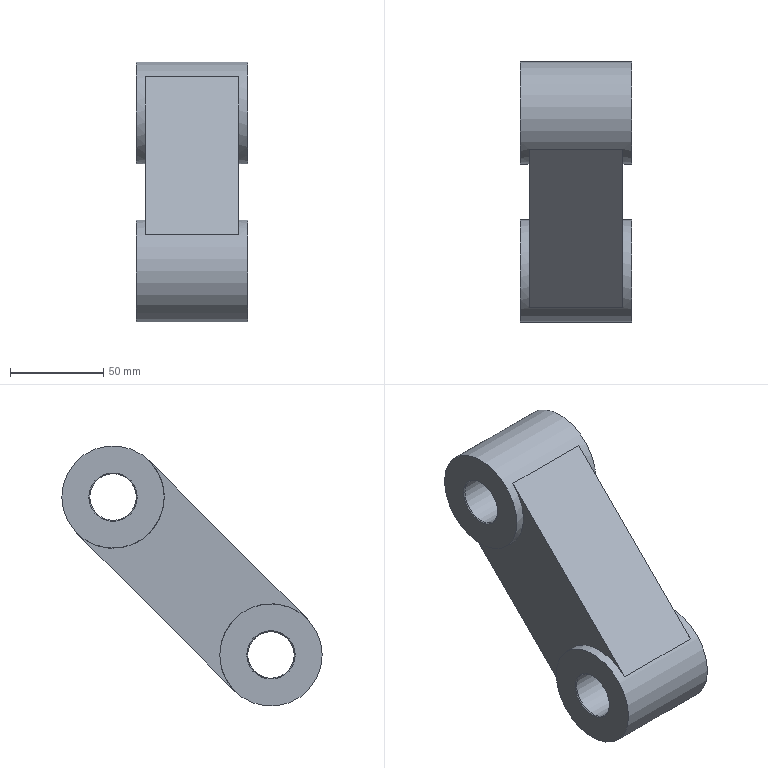Part | NX | features solid 2 | 1 solid | 19 faces | box 60 x 139.853 x 139.853 mm | volume 437363 mm3 | plane 8 | cone 7 | cylinder 4 | commonest cylinder face diameters 25 x2 55 x2
STEP:
#1=CARTESIAN_POINT('',(525.,-759.445,-230.555));
#2=VERTEX_POINT('',#1);
#3=CARTESIAN_POINT('',(475.,-759.445,-230.555));
#4=VERTEX_POINT('',#3);
#5=CARTESIAN_POINT('',(525.,-759.445,-230.555));
#6=DIRECTION('',(-1.,0.,0.));
#7=VECTOR('',#6,1000.);
#8=LINE('',#5,#7);
#9=EDGE_CURVE('',#2,#4,#8,.T.);
#10=ORIENTED_EDGE('',*,*,#9,.F.);
#11=CARTESIAN_POINT('',(525.,-674.593,-145.702));
#12=VERTEX_POINT('',#11);
#13=CARTESIAN_POINT('',(525.,-759.445,-230.555));
#14=DIRECTION('',(0.,0.7071,0.7071));
#15=VECTOR('',#14,1000.);
#16=LINE('',#13,#15);
#17=EDGE_CURVE('',#2,#12,#16,.T.);
#18=ORIENTED_EDGE('',*,*,#17,.T.);
#19=CARTESIAN_POINT('',(475.,-674.593,-145.702));
#20=VERTEX_POINT('',#19);
#21=CARTESIAN_POINT('',(525.,-674.593,-145.702));
#22=DIRECTION('',(-1.,0.,0.));
#23=VECTOR('',#22,1000.);
#24=LINE('',#21,#23);
#25=EDGE_CURVE('',#12,#20,#24,.T.);
#26=ORIENTED_EDGE('',*,*,#25,.T.);
#27=CARTESIAN_POINT('',(475.,-717.019,-188.128));
#28=DIRECTION('',(0.,0.7071,0.7071));
#29=VECTOR('',#28,1000.);
#30=LINE('',#27,#29);
#31=EDGE_CURVE('',#4,#20,#30,.T.);
#32=ORIENTED_EDGE('',*,*,#31,.F.);
#33=EDGE_LOOP('',(#10,#18,#26,#32));
#34=FACE_BOUND('',#33,.T.);
#35=CARTESIAN_POINT('',(575.,-778.891,-250.));
#36=DIRECTION('',(0.,-0.7071,0.7071));
#37=DIRECTION('',(0.,0.7071,0.7071));
#38=AXIS2_PLACEMENT_3D('',#35,#36,#37);
#39=PLANE('',#38);
#40=ADVANCED_FACE('',(#34),#39,.T.);
#41=CARTESIAN_POINT('',(470.,-712.5,-250.));
#42=VERTEX_POINT('',#41);
#43=CARTESIAN_POINT('',(470.,-740.,-250.));
#44=DIRECTION('',(1.,0.,0.));
#45=DIRECTION('',(0.,1.,0.));
#46=AXIS2_PLACEMENT_3D('',#43,#44,#45);
#47=CIRCLE('',#46,27.5);
#48=EDGE_CURVE('',#42,#42,#47,.T.);
#49=ORIENTED_EDGE('',*,*,#48,.T.);
#50=EDGE_LOOP('',(#49));
#51=FACE_BOUND('',#50,.T.);
#52=CARTESIAN_POINT('',(530.,-712.5,-250.));
#53=VERTEX_POINT('',#52);
#54=CARTESIAN_POINT('',(530.,-740.,-250.));
#55=DIRECTION('',(1.,0.,0.));
#56=DIRECTION('',(0.,1.,0.));
#57=AXIS2_PLACEMENT_3D('',#54,#55,#56);
#58=CIRCLE('',#57,27.5);
#59=EDGE_CURVE('',#53,#53,#58,.T.);
#60=ORIENTED_EDGE('',*,*,#59,.F.);
#61=EDGE_LOOP('',(#60));
#62=FACE_BOUND('',#61,.T.);
#63=CARTESIAN_POINT('',(475.,-720.555,-269.445));
#64=VERTEX_POINT('',#63);
#65=CARTESIAN_POINT('',(475.,-740.,-250.));
#66=DIRECTION('',(1.,0.,0.));
#67=DIRECTION('',(0.,1.,0.));
#68=AXIS2_PLACEMENT_3D('',#65,#66,#67);
#69=CIRCLE('',#68,27.5);
#70=EDGE_CURVE('',#64,#4,#69,.T.);
#71=ORIENTED_EDGE('',*,*,#70,.F.);
#72=CARTESIAN_POINT('',(525.,-720.555,-269.445));
#73=VERTEX_POINT('',#72);
#74=CARTESIAN_POINT('',(500.005,-720.555,-269.445));
#75=DIRECTION('',(-1.,0.,0.));
#76=VECTOR('',#75,1000.);
#77=LINE('',#74,#76);
#78=EDGE_CURVE('',#73,#64,#77,.T.);
#79=ORIENTED_EDGE('',*,*,#78,.F.);
#80=CARTESIAN_POINT('',(525.,-740.,-250.));
#81=DIRECTION('',(-1.,0.,0.));
#82=DIRECTION('',(0.,1.,0.));
#83=AXIS2_PLACEMENT_3D('',#80,#81,#82);
#84=CIRCLE('',#83,27.5);
#85=EDGE_CURVE('',#2,#73,#84,.T.);
#86=ORIENTED_EDGE('',*,*,#85,.F.);
#87=ORIENTED_EDGE('',*,*,#9,.T.);
#88=EDGE_LOOP('',(#71,#79,#86,#87));
#89=FACE_BOUND('',#88,.T.);
#90=CARTESIAN_POINT('',(530.106,-740.,-250.));
#91=DIRECTION('',(-1.,0.,0.));
#92=DIRECTION('',(0.,0.,-1.));
#93=AXIS2_PLACEMENT_3D('',#90,#91,#92);
#94=CYLINDRICAL_SURFACE('',#93,27.5);
#95=ADVANCED_FACE('',(#51,#62,#89),#94,.T.);
#96=CARTESIAN_POINT('',(525.,-635.702,-184.593));
#97=VERTEX_POINT('',#96);
#98=CARTESIAN_POINT('',(525.,-678.128,-227.019));
#99=DIRECTION('',(0.,-0.7071,-0.7071));
#100=VECTOR('',#99,1000.);
#101=LINE('',#98,#100);
#102=EDGE_CURVE('',#97,#73,#101,.T.);
#103=ORIENTED_EDGE('',*,*,#102,.T.);
#104=ORIENTED_EDGE('',*,*,#78,.T.);
#105=CARTESIAN_POINT('',(475.,-635.702,-184.593));
#106=VERTEX_POINT('',#105);
#107=CARTESIAN_POINT('',(475.,-678.128,-227.019));
#108=DIRECTION('',(0.,-0.7071,-0.7071));
#109=VECTOR('',#108,1000.);
#110=LINE('',#107,#109);
#111=EDGE_CURVE('',#106,#64,#110,.T.);
#112=ORIENTED_EDGE('',*,*,#111,.F.);
#113=CARTESIAN_POINT('',(500.,-635.702,-184.593));
#114=DIRECTION('',(-1.,0.,0.));
#115=VECTOR('',#114,1000.);
#116=LINE('',#113,#115);
#117=EDGE_CURVE('',#97,#106,#116,.T.);
#118=ORIENTED_EDGE('',*,*,#117,.F.);
#119=EDGE_LOOP('',(#103,#104,#112,#118));
#120=FACE_BOUND('',#119,.T.);
#121=CARTESIAN_POINT('',(575.,-616.256,-165.147));
#122=DIRECTION('',(0.,0.7071,-0.7071));
#123=DIRECTION('',(0.,-0.7071,-0.7071));
#124=AXIS2_PLACEMENT_3D('',#121,#122,#123);
#125=PLANE('',#124);
#126=ADVANCED_FACE('',(#120),#125,.T.);
#127=CARTESIAN_POINT('',(525.,-655.147,-165.147));
#128=DIRECTION('',(-1.,0.,0.));
#129=DIRECTION('',(0.,1.,0.));
#130=AXIS2_PLACEMENT_3D('',#127,#128,#129);
#131=CIRCLE('',#130,27.5);
#132=EDGE_CURVE('',#97,#12,#131,.T.);
#133=ORIENTED_EDGE('',*,*,#132,.F.);
#134=ORIENTED_EDGE('',*,*,#117,.T.);
#135=CARTESIAN_POINT('',(475.,-655.147,-165.147));
#136=DIRECTION('',(1.,0.,0.));
#137=DIRECTION('',(0.,1.,0.));
#138=AXIS2_PLACEMENT_3D('',#135,#136,#137);
#139=CIRCLE('',#138,27.5);
#140=EDGE_CURVE('',#20,#106,#139,.T.);
#141=ORIENTED_EDGE('',*,*,#140,.F.);
#142=ORIENTED_EDGE('',*,*,#25,.F.);
#143=EDGE_LOOP('',(#133,#134,#141,#142));
#144=FACE_BOUND('',#143,.T.);
#145=CARTESIAN_POINT('',(470.,-627.647,-165.147));
#146=VERTEX_POINT('',#145);
#147=CARTESIAN_POINT('',(470.,-655.147,-165.147));
#148=DIRECTION('',(1.,0.,0.));
#149=DIRECTION('',(0.,1.,0.));
#150=AXIS2_PLACEMENT_3D('',#147,#148,#149);
#151=CIRCLE('',#150,27.5);
#152=EDGE_CURVE('',#146,#146,#151,.T.);
#153=ORIENTED_EDGE('',*,*,#152,.T.);
#154=EDGE_LOOP('',(#153));
#155=FACE_BOUND('',#154,.T.);
#156=CARTESIAN_POINT('',(530.,-627.647,-165.147));
#157=VERTEX_POINT('',#156);
#158=CARTESIAN_POINT('',(530.,-655.147,-165.147));
#159=DIRECTION('',(1.,0.,0.));
#160=DIRECTION('',(0.,1.,0.));
#161=AXIS2_PLACEMENT_3D('',#158,#159,#160);
#162=CIRCLE('',#161,27.5);
#163=EDGE_CURVE('',#157,#157,#162,.T.);
#164=ORIENTED_EDGE('',*,*,#163,.F.);
#165=EDGE_LOOP('',(#164));
#166=FACE_BOUND('',#165,.T.);
#167=CARTESIAN_POINT('',(530.106,-655.147,-165.147));
#168=DIRECTION('',(-1.,0.,0.));
#169=DIRECTION('',(0.,0.,-1.));
#170=AXIS2_PLACEMENT_3D('',#167,#168,#169);
#171=CYLINDRICAL_SURFACE('',#170,27.5);
#172=ADVANCED_FACE('',(#144,#155,#166),#171,.T.);
#173=ORIENTED_EDGE('',*,*,#17,.F.);
#174=ORIENTED_EDGE('',*,*,#85,.T.);
#175=ORIENTED_EDGE('',*,*,#102,.F.);
#176=ORIENTED_EDGE('',*,*,#132,.T.);
#177=EDGE_LOOP('',(#173,#174,#175,#176));
#178=FACE_BOUND('',#177,.T.);
#179=CARTESIAN_POINT('',(525.,-707.705,-134.764));
#180=DIRECTION('',(-1.,0.,0.));
#181=DIRECTION('',(0.,0.,-1.));
#182=AXIS2_PLACEMENT_3D('',#179,#180,#181);
#183=PLANE('',#182);
#184=ADVANCED_FACE('',(#178),#183,.F.);
#185=ORIENTED_EDGE('',*,*,#48,.F.);
#186=EDGE_LOOP('',(#185));
#187=FACE_BOUND('',#186,.T.);
#188=CARTESIAN_POINT('',(470.,-727.,-250.));
#189=VERTEX_POINT('',#188);
#190=CARTESIAN_POINT('',(470.,-753.,-250.));
#191=VERTEX_POINT('',#190);
#192=CARTESIAN_POINT('',(470.,-740.,-250.));
#193=DIRECTION('',(1.,0.,0.));
#194=DIRECTION('',(0.,0.,-1.));
#195=AXIS2_PLACEMENT_3D('',#192,#193,#194);
#196=CIRCLE('',#195,13.);
#197=EDGE_CURVE('',#189,#191,#196,.T.);
#198=ORIENTED_EDGE('',*,*,#197,.T.);
#199=CARTESIAN_POINT('',(470.,-740.,-250.));
#200=DIRECTION('',(1.,0.,0.));
#201=DIRECTION('',(0.,0.,-1.));
#202=AXIS2_PLACEMENT_3D('',#199,#200,#201);
#203=CIRCLE('',#202,13.);
#204=EDGE_CURVE('',#191,#189,#203,.T.);
#205=ORIENTED_EDGE('',*,*,#204,.T.);
#206=EDGE_LOOP('',(#198,#205));
#207=FACE_BOUND('',#206,.T.);
#208=CARTESIAN_POINT('',(470.,-743.7,-355.311));
#209=DIRECTION('',(-1.,0.,0.));
#210=DIRECTION('',(0.,0.,-1.));
#211=AXIS2_PLACEMENT_3D('',#208,#209,#210);
#212=PLANE('',#211);
#213=ADVANCED_FACE('',(#187,#207),#212,.T.);
#214=CARTESIAN_POINT('',(470.5,-727.5,-250.));
#215=VERTEX_POINT('',#214);
#216=CARTESIAN_POINT('',(470.244,-727.244,-250.));
#217=DIRECTION('',(-0.7071,0.7071,0.));
#218=VECTOR('',#217,1000.);
#219=LINE('',#216,#218);
#220=EDGE_CURVE('',#215,#189,#219,.T.);
#221=ORIENTED_EDGE('',*,*,#220,.F.);
#222=CARTESIAN_POINT('',(470.5,-752.5,-250.));
#223=VERTEX_POINT('',#222);
#224=CARTESIAN_POINT('',(470.5,-740.,-250.));
#225=DIRECTION('',(-1.,0.,0.));
#226=DIRECTION('',(0.,0.,1.));
#227=AXIS2_PLACEMENT_3D('',#224,#225,#226);
#228=CIRCLE('',#227,12.5);
#229=EDGE_CURVE('',#215,#223,#228,.F.);
#230=ORIENTED_EDGE('',*,*,#229,.T.);
#231=CARTESIAN_POINT('',(470.244,-752.756,-250.));
#232=DIRECTION('',(-0.7071,-0.7071,0.));
#233=VECTOR('',#232,1000.);
#234=LINE('',#231,#233);
#235=EDGE_CURVE('',#191,#223,#234,.F.);
#236=ORIENTED_EDGE('',*,*,#235,.F.);
#237=ORIENTED_EDGE('',*,*,#197,.F.);
#238=EDGE_LOOP('',(#221,#230,#236,#237));
#239=FACE_BOUND('',#238,.T.);
#240=CARTESIAN_POINT('',(470.566,-740.,-250.));
#241=DIRECTION('',(-1.,0.,0.));
#242=DIRECTION('',(0.,0.,-1.));
#243=AXIS2_PLACEMENT_3D('',#240,#241,#242);
#244=CONICAL_SURFACE('',#243,12.434,0.7854);
#245=ADVANCED_FACE('',(#239),#244,.F.);
#246=CARTESIAN_POINT('',(470.5,-740.,-250.));
#247=DIRECTION('',(-1.,0.,0.));
#248=DIRECTION('',(0.,0.,1.));
#249=AXIS2_PLACEMENT_3D('',#246,#247,#248);
#250=CIRCLE('',#249,12.5);
#251=EDGE_CURVE('',#223,#215,#250,.F.);
#252=ORIENTED_EDGE('',*,*,#251,.T.);
#253=ORIENTED_EDGE('',*,*,#220,.T.);
#254=ORIENTED_EDGE('',*,*,#204,.F.);
#255=ORIENTED_EDGE('',*,*,#235,.T.);
#256=EDGE_LOOP('',(#252,#253,#254,#255));
#257=FACE_BOUND('',#256,.T.);
#258=CARTESIAN_POINT('',(470.566,-740.,-250.));
#259=DIRECTION('',(-1.,0.,0.));
#260=DIRECTION('',(0.,0.,-1.));
#261=AXIS2_PLACEMENT_3D('',#258,#259,#260);
#262=CONICAL_SURFACE('',#261,12.434,0.7854);
#263=ADVANCED_FACE('',(#257),#262,.F.);
#264=ORIENTED_EDGE('',*,*,#31,.T.);
#265=ORIENTED_EDGE('',*,*,#140,.T.);
#266=ORIENTED_EDGE('',*,*,#111,.T.);
#267=ORIENTED_EDGE('',*,*,#70,.T.);
#268=EDGE_LOOP('',(#264,#265,#266,#267));
#269=FACE_BOUND('',#268,.T.);
#270=CARTESIAN_POINT('',(475.,-707.705,-134.764));
#271=DIRECTION('',(-1.,0.,0.));
#272=DIRECTION('',(0.,0.,-1.));
#273=AXIS2_PLACEMENT_3D('',#270,#271,#272);
#274=PLANE('',#273);
#275=ADVANCED_FACE('',(#269),#274,.T.);
#276=ORIENTED_EDGE('',*,*,#163,.T.);
#277=EDGE_LOOP('',(#276));
#278=FACE_BOUND('',#277,.T.);
#279=CARTESIAN_POINT('',(530.,-668.147,-165.147));
#280=VERTEX_POINT('',#279);
#281=CARTESIAN_POINT('',(530.,-642.147,-165.147));
#282=VERTEX_POINT('',#281);
#283=CARTESIAN_POINT('',(530.,-655.147,-165.147));
#284=DIRECTION('',(-1.,0.,0.));
#285=DIRECTION('',(0.,0.,1.));
#286=AXIS2_PLACEMENT_3D('',#283,#284,#285);
#287=CIRCLE('',#286,13.);
#288=EDGE_CURVE('',#280,#282,#287,.T.);
#289=ORIENTED_EDGE('',*,*,#288,.T.);
#290=CARTESIAN_POINT('',(530.,-655.147,-165.147));
#291=DIRECTION('',(-1.,0.,0.));
#292=DIRECTION('',(0.,0.,1.));
#293=AXIS2_PLACEMENT_3D('',#290,#291,#292);
#294=CIRCLE('',#293,13.);
#295=EDGE_CURVE('',#282,#280,#294,.T.);
#296=ORIENTED_EDGE('',*,*,#295,.T.);
#297=EDGE_LOOP('',(#289,#296));
#298=FACE_BOUND('',#297,.T.);
#299=CARTESIAN_POINT('',(530.,-658.847,-59.836));
#300=DIRECTION('',(1.,0.,0.));
#301=DIRECTION('',(0.,0.,1.));
#302=AXIS2_PLACEMENT_3D('',#299,#300,#301);
#303=PLANE('',#302);
#304=ADVANCED_FACE('',(#278,#298),#303,.T.);
#305=ORIENTED_EDGE('',*,*,#59,.T.);
#306=EDGE_LOOP('',(#305));
#307=FACE_BOUND('',#306,.T.);
#308=CARTESIAN_POINT('',(530.,-740.,-237.));
#309=VERTEX_POINT('',#308);
#310=CARTESIAN_POINT('',(530.,-740.,-250.));
#311=DIRECTION('',(-1.,0.,0.));
#312=DIRECTION('',(0.,0.,1.));
#313=AXIS2_PLACEMENT_3D('',#310,#311,#312);
#314=CIRCLE('',#313,13.);
#315=EDGE_CURVE('',#309,#309,#314,.T.);
#316=ORIENTED_EDGE('',*,*,#315,.T.);
#317=EDGE_LOOP('',(#316));
#318=FACE_BOUND('',#317,.T.);
#319=CARTESIAN_POINT('',(530.,-743.7,-144.689));
#320=DIRECTION('',(1.,0.,0.));
#321=DIRECTION('',(0.,0.,1.));
#322=AXIS2_PLACEMENT_3D('',#319,#320,#321);
#323=PLANE('',#322);
#324=ADVANCED_FACE('',(#307,#318),#323,.T.);
#325=ORIENTED_EDGE('',*,*,#152,.F.);
#326=EDGE_LOOP('',(#325));
#327=FACE_BOUND('',#326,.T.);
#328=CARTESIAN_POINT('',(470.,-668.147,-165.147));
#329=VERTEX_POINT('',#328);
#330=CARTESIAN_POINT('',(470.,-642.147,-165.147));
#331=VERTEX_POINT('',#330);
#332=CARTESIAN_POINT('',(470.,-655.147,-165.147));
#333=DIRECTION('',(1.,0.,0.));
#334=DIRECTION('',(0.,0.,-1.));
#335=AXIS2_PLACEMENT_3D('',#332,#333,#334);
#336=CIRCLE('',#335,13.);
#337=EDGE_CURVE('',#329,#331,#336,.T.);
#338=ORIENTED_EDGE('',*,*,#337,.T.);
#339=CARTESIAN_POINT('',(470.,-655.147,-165.147));
#340=DIRECTION('',(1.,0.,0.));
#341=DIRECTION('',(0.,0.,-1.));
#342=AXIS2_PLACEMENT_3D('',#339,#340,#341);
#343=CIRCLE('',#342,13.);
#344=EDGE_CURVE('',#331,#329,#343,.T.);
#345=ORIENTED_EDGE('',*,*,#344,.T.);
#346=EDGE_LOOP('',(#338,#345));
#347=FACE_BOUND('',#346,.T.);
#348=CARTESIAN_POINT('',(470.,-658.847,-270.459));
#349=DIRECTION('',(-1.,0.,0.));
#350=DIRECTION('',(0.,0.,-1.));
#351=AXIS2_PLACEMENT_3D('',#348,#349,#350);
#352=PLANE('',#351);
#353=ADVANCED_FACE('',(#327,#347),#352,.T.);
#354=CARTESIAN_POINT('',(529.5,-727.5,-250.));
#355=VERTEX_POINT('',#354);
#356=CARTESIAN_POINT('',(529.5,-740.,-250.));
#357=DIRECTION('',(-1.,0.,0.));
#358=DIRECTION('',(0.,1.,0.));
#359=AXIS2_PLACEMENT_3D('',#356,#357,#358);
#360=CIRCLE('',#359,12.5);
#361=EDGE_CURVE('',#355,#355,#360,.T.);
#362=ORIENTED_EDGE('',*,*,#361,.F.);
#363=EDGE_LOOP('',(#362));
#364=FACE_BOUND('',#363,.T.);
#365=ORIENTED_EDGE('',*,*,#251,.F.);
#366=ORIENTED_EDGE('',*,*,#229,.F.);
#367=EDGE_LOOP('',(#365,#366));
#368=FACE_BOUND('',#367,.T.);
#369=CARTESIAN_POINT('',(470.096,-740.,-250.));
#370=DIRECTION('',(1.,0.,0.));
#371=DIRECTION('',(0.,0.,1.));
#372=AXIS2_PLACEMENT_3D('',#369,#370,#371);
#373=CYLINDRICAL_SURFACE('',#372,12.5);
#374=ADVANCED_FACE('',(#364,#368),#373,.F.);
#375=CARTESIAN_POINT('',(470.5,-642.647,-165.147));
#376=VERTEX_POINT('',#375);
#377=CARTESIAN_POINT('',(470.5,-667.647,-165.147));
#378=VERTEX_POINT('',#377);
#379=CARTESIAN_POINT('',(470.5,-655.147,-165.147));
#380=DIRECTION('',(1.,0.,0.));
#381=DIRECTION('',(0.,1.,0.));
#382=AXIS2_PLACEMENT_3D('',#379,#380,#381);
#383=CIRCLE('',#382,12.5);
#384=EDGE_CURVE('',#376,#378,#383,.T.);
#385=ORIENTED_EDGE('',*,*,#384,.F.);
#386=CARTESIAN_POINT('',(470.5,-655.147,-165.147));
#387=DIRECTION('',(1.,0.,0.));
#388=DIRECTION('',(0.,1.,0.));
#389=AXIS2_PLACEMENT_3D('',#386,#387,#388);
#390=CIRCLE('',#389,12.5);
#391=EDGE_CURVE('',#378,#376,#390,.T.);
#392=ORIENTED_EDGE('',*,*,#391,.F.);
#393=EDGE_LOOP('',(#385,#392));
#394=FACE_BOUND('',#393,.T.);
#395=CARTESIAN_POINT('',(529.5,-642.647,-165.147));
#396=VERTEX_POINT('',#395);
#397=CARTESIAN_POINT('',(529.5,-667.647,-165.147));
#398=VERTEX_POINT('',#397);
#399=CARTESIAN_POINT('',(529.5,-655.147,-165.147));
#400=DIRECTION('',(-1.,0.,0.));
#401=DIRECTION('',(0.,1.,0.));
#402=AXIS2_PLACEMENT_3D('',#399,#400,#401);
#403=CIRCLE('',#402,12.5);
#404=EDGE_CURVE('',#396,#398,#403,.T.);
#405=ORIENTED_EDGE('',*,*,#404,.F.);
#406=CARTESIAN_POINT('',(529.5,-655.147,-165.147));
#407=DIRECTION('',(-1.,0.,0.));
#408=DIRECTION('',(0.,1.,0.));
#409=AXIS2_PLACEMENT_3D('',#406,#407,#408);
#410=CIRCLE('',#409,12.5);
#411=EDGE_CURVE('',#398,#396,#410,.T.);
#412=ORIENTED_EDGE('',*,*,#411,.F.);
#413=EDGE_LOOP('',(#405,#412));
#414=FACE_BOUND('',#413,.T.);
#415=CARTESIAN_POINT('',(529.915,-655.147,-165.147));
#416=DIRECTION('',(-1.,0.,0.));
#417=DIRECTION('',(0.,0.,-1.));
#418=AXIS2_PLACEMENT_3D('',#415,#416,#417);
#419=CYLINDRICAL_SURFACE('',#418,12.5);
#420=ADVANCED_FACE('',(#394,#414),#419,.F.);
#421=CARTESIAN_POINT('',(529.749,-642.398,-165.147));
#422=DIRECTION('',(0.7071,0.7071,0.));
#423=VECTOR('',#422,1000.);
#424=LINE('',#421,#423);
#425=EDGE_CURVE('',#396,#282,#424,.T.);
#426=ORIENTED_EDGE('',*,*,#425,.T.);
#427=ORIENTED_EDGE('',*,*,#288,.F.);
#428=CARTESIAN_POINT('',(529.749,-667.896,-165.147));
#429=DIRECTION('',(0.7071,-0.7071,0.));
#430=VECTOR('',#429,1000.);
#431=LINE('',#428,#430);
#432=EDGE_CURVE('',#280,#398,#431,.F.);
#433=ORIENTED_EDGE('',*,*,#432,.T.);
#434=ORIENTED_EDGE('',*,*,#411,.T.);
#435=EDGE_LOOP('',(#426,#427,#433,#434));
#436=FACE_BOUND('',#435,.T.);
#437=CARTESIAN_POINT('',(529.427,-655.147,-165.147));
#438=DIRECTION('',(1.,0.,0.));
#439=DIRECTION('',(0.,0.,1.));
#440=AXIS2_PLACEMENT_3D('',#437,#438,#439);
#441=CONICAL_SURFACE('',#440,12.427,0.7854);
#442=ADVANCED_FACE('',(#436),#441,.F.);
#443=ORIENTED_EDGE('',*,*,#315,.F.);
#444=EDGE_LOOP('',(#443));
#445=FACE_BOUND('',#444,.T.);
#446=ORIENTED_EDGE('',*,*,#361,.T.);
#447=EDGE_LOOP('',(#446));
#448=FACE_BOUND('',#447,.T.);
#449=CARTESIAN_POINT('',(529.429,-740.,-250.));
#450=DIRECTION('',(1.,0.,0.));
#451=DIRECTION('',(0.,0.,1.));
#452=AXIS2_PLACEMENT_3D('',#449,#450,#451);
#453=CONICAL_SURFACE('',#452,12.429,0.7854);
#454=ADVANCED_FACE('',(#445,#448),#453,.F.);
#455=CARTESIAN_POINT('',(470.244,-667.903,-165.147));
#456=DIRECTION('',(-0.7071,-0.7071,0.));
#457=VECTOR('',#456,1000.);
#458=LINE('',#455,#457);
#459=EDGE_CURVE('',#378,#329,#458,.T.);
#460=ORIENTED_EDGE('',*,*,#459,.F.);
#461=ORIENTED_EDGE('',*,*,#391,.T.);
#462=CARTESIAN_POINT('',(470.244,-642.392,-165.147));
#463=DIRECTION('',(-0.7071,0.7071,0.));
#464=VECTOR('',#463,1000.);
#465=LINE('',#462,#464);
#466=EDGE_CURVE('',#331,#376,#465,.F.);
#467=ORIENTED_EDGE('',*,*,#466,.F.);
#468=ORIENTED_EDGE('',*,*,#337,.F.);
#469=EDGE_LOOP('',(#460,#461,#467,#468));
#470=FACE_BOUND('',#469,.T.);
#471=CARTESIAN_POINT('',(470.566,-655.147,-165.147));
#472=DIRECTION('',(-1.,0.,0.));
#473=DIRECTION('',(0.,0.,-1.));
#474=AXIS2_PLACEMENT_3D('',#471,#472,#473);
#475=CONICAL_SURFACE('',#474,12.434,0.7854);
#476=ADVANCED_FACE('',(#470),#475,.F.);
#477=ORIENTED_EDGE('',*,*,#295,.F.);
#478=ORIENTED_EDGE('',*,*,#425,.F.);
#479=ORIENTED_EDGE('',*,*,#404,.T.);
#480=ORIENTED_EDGE('',*,*,#432,.F.);
#481=EDGE_LOOP('',(#477,#478,#479,#480));
#482=FACE_BOUND('',#481,.T.);
#483=CARTESIAN_POINT('',(529.427,-655.147,-165.147));
#484=DIRECTION('',(1.,0.,0.));
#485=DIRECTION('',(0.,0.,1.));
#486=AXIS2_PLACEMENT_3D('',#483,#484,#485);
#487=CONICAL_SURFACE('',#486,12.427,0.7854);
#488=ADVANCED_FACE('',(#482),#487,.F.);
#489=ORIENTED_EDGE('',*,*,#344,.F.);
#490=ORIENTED_EDGE('',*,*,#466,.T.);
#491=ORIENTED_EDGE('',*,*,#384,.T.);
#492=ORIENTED_EDGE('',*,*,#459,.T.);
#493=EDGE_LOOP('',(#489,#490,#491,#492));
#494=FACE_BOUND('',#493,.T.);
#495=CARTESIAN_POINT('',(470.566,-655.147,-165.147));
#496=DIRECTION('',(-1.,0.,0.));
#497=DIRECTION('',(0.,0.,-1.));
#498=AXIS2_PLACEMENT_3D('',#495,#496,#497);
#499=CONICAL_SURFACE('',#498,12.434,0.7854);
#500=ADVANCED_FACE('',(#494),#499,.F.);
#501=CLOSED_SHELL('',(#40,#95,#126,#172,#184,#213,#245,#263,#275,#304,#324,#353,#374,#420,#442,#454,#476,#488,#500));
#502=MANIFOLD_SOLID_BREP('',#501);
#503=(LENGTH_UNIT()NAMED_UNIT(*)SI_UNIT(.MILLI.,.METRE.));
#504=UNCERTAINTY_MEASURE_WITH_UNIT(LENGTH_MEASURE(0.00001),#503,'','');
#505=(NAMED_UNIT(*)PLANE_ANGLE_UNIT()SI_UNIT($,.RADIAN.));
#506=(NAMED_UNIT(*)SI_UNIT($,.STERADIAN.)SOLID_ANGLE_UNIT());
#507=(GEOMETRIC_REPRESENTATION_CONTEXT(3)GLOBAL_UNCERTAINTY_ASSIGNED_CONTEXT((#504))GLOBAL_UNIT_ASSIGNED_CONTEXT((#503,#505,#506))REPRESENTATION_CONTEXT('',''));
#508=ADVANCED_BREP_SHAPE_REPRESENTATION('',(#502),#507);